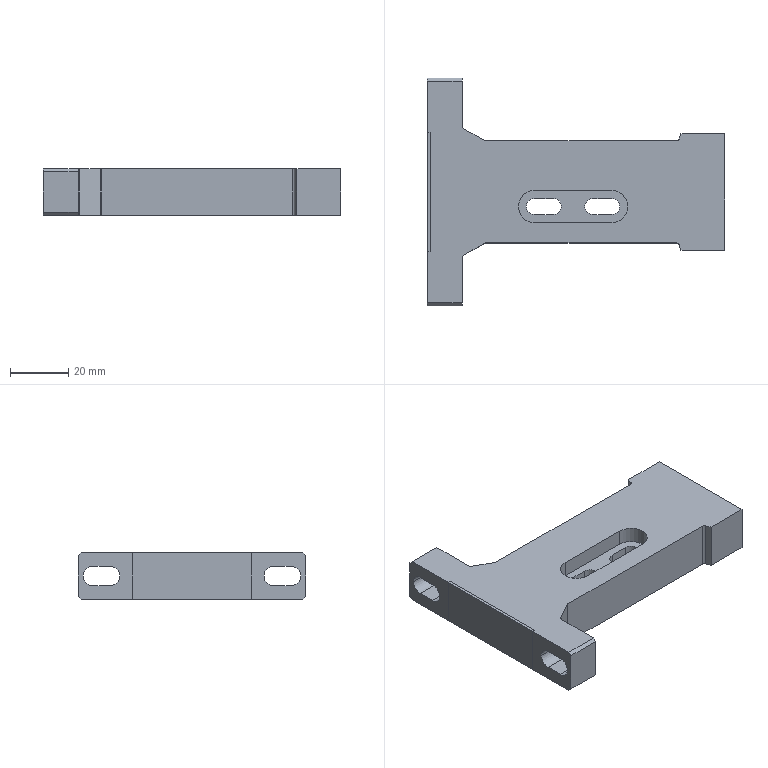NC program | NX | posted with a generic post | part box 102 x 78 x 16 mm
Lines 2465 to 2749 of 11044:
(ZLEVEL_PROFILE_COPY_COPY_1 , TOOL : D10JING)
N4922 T11 M6
N4924 G54
N4926 G17 G0 G90 X-56.438 Y-39.827 B0. C0. S9500 M3
N4928 G43 Z30. H11
N4930 Z-13.
N4932 G94 G1 Z-16. F1200.
N4934 G3 X-56. Y-39. R1.
N4936 G1 Y39.
N4938 G2 X-51. Y44. R5.
N4940 G1 X-39.
N4942 G2 X-34. Y39. R5.
N4944 G1 Y24.887
N4946 X-29.866 Y22.5
N4948 X31.67
N4950 G2 X36. Y25. R5.
N4952 G1 X51.
N4954 G2 X56. Y20. R5.
N4956 G1 Y-20.
N4958 G2 X51. Y-25. R5.
N4960 G1 X36.
N4962 G2 X31.67 Y-22.5 R5.
N4964 G1 X-29.866
N4966 X-34. Y-24.887
N4968 Y-39.
N4970 G2 X-39. Y-44. R5.
N4972 G1 X-51.
N4974 G2 X-56. Y-39. R5.
N4976 G3 X-56.5 Y-38.134 R1.
N4978 G1 Z-13.
N4980 G0 Z30.
N4982 M5
(ZLEVEL_PROFILE_COPY_COPY_1_COPY_1 , TOOL : D6)
N4984 T06 M6
N4986 G54
N4988 G17 G0 G90 X14.695 Y-5.095 B0. C0. S9500 M3
N4990 G43 Z30. H6
N4992 Z1.5
N4994 G94 G1 X14.691 Y-4.699 Z1.479 F2200.
N4996 X14.559 Y-4.152 Z1.45
N4998 X14.37 Y-3.752 Z1.427
N5000 X14.017 Y-3.289 Z1.396
N5002 X13.566 Y-2.921 Z1.366
N5004 X13.041 Y-2.671 Z1.335
N5006 X12.472 Y-2.55 Z1.305
N5008 X-14.472 Z-0.107
N5010 X-15.041 Y-2.671 Z-0.138
N5012 X-15.566 Y-2.921 Z-0.168
N5014 X-16.017 Y-3.289 Z-0.199
N5016 X-16.37 Y-3.752 Z-0.229
N5018 X-16.559 Y-4.152 Z-0.253
N5020 X-16.691 Y-4.699 Z-0.282
N5022 X-16.696 Y-5.261 Z-0.312
N5024 X-16.573 Y-5.809 Z-0.341
N5026 X-16.329 Y-6.316 Z-0.371
N5028 X-15.975 Y-6.753 Z-0.4
N5030 X-15.532 Y-7.099 Z-0.429
N5032 X-15.022 Y-7.336 Z-0.459
N5034 X-14.472 Y-7.45 Z-0.488
N5036 X-14.25 Z-0.5
N5038 X12.25
N5040 G3 X14.7 Y-5. R2.45
N5042 X12.25 Y-2.55 R2.45
N5044 G1 X-14.25
N5046 G3 X-16.7 Y-5. R2.45
N5048 X-14.25 Y-7.45 R2.45
N5050 G1 X11.979 Z-0.958
N5052 X12.152 Z-0.961
N5054 X12.324 Y-7.44 Z-0.964
N5056 X12.496 Y-7.431 Z-0.967
N5058 X12.666 Y-7.406 Z-0.97
N5060 X12.835 Y-7.373 Z-0.973
N5062 X13. Y-7.324 Z-0.976
N5064 X13.162 Y-7.266 Z-0.979
N5066 X13.32 Y-7.198 Z-0.982
N5068 X13.47 Y-7.114 Z-0.985
N5070 X13.618 Y-7.026 Z-0.988
N5072 X13.755 Y-6.923 Z-0.991
N5074 X13.887 Y-6.812 Z-0.994
N5076 X14.012 Y-6.693 Z-0.997
N5078 X14.131 Y-6.569 Z-1.
N5080 G3 X12.25 Y-2.55 R2.45
N5082 G1 X-14.25
N5084 G3 X-16.7 Y-5. R2.45
N5086 X-14.25 Y-7.45 R2.45
N5088 G1 X11.979 Z-1.458
N5090 X12.152 Z-1.461
N5092 X12.324 Y-7.44 Z-1.464
N5094 X12.496 Y-7.431 Z-1.467
N5096 X12.666 Y-7.406 Z-1.47
N5098 X12.835 Y-7.373 Z-1.473
N5100 X13. Y-7.323 Z-1.476
N5102 X13.161 Y-7.265 Z-1.479
N5104 X13.319 Y-7.198 Z-1.482
N5106 X13.47 Y-7.114 Z-1.485
N5108 X13.617 Y-7.026 Z-1.488
N5110 X13.755 Y-6.923 Z-1.491
N5112 X13.886 Y-6.812 Z-1.494
N5114 X14.012 Y-6.693 Z-1.497
N5116 X14.131 Y-6.569 Z-1.5
N5118 G3 X12.25 Y-2.55 R2.45
N5120 G1 X-14.25
N5122 G3 X-16.7 Y-5. R2.45
N5124 X-14.25 Y-7.45 R2.45
N5126 G1 X11.979 Z-1.958
N5128 X12.152 Z-1.961
N5130 X12.324 Y-7.44 Z-1.964
N5132 X12.496 Y-7.431 Z-1.967
N5134 X12.666 Y-7.406 Z-1.97
N5136 X12.835 Y-7.372 Z-1.973
N5138 X12.999 Y-7.323 Z-1.976
N5140 X13.161 Y-7.265 Z-1.979
N5142 X13.319 Y-7.198 Z-1.982
N5144 X13.47 Y-7.114 Z-1.985
N5146 X13.617 Y-7.026 Z-1.988
N5148 X13.755 Y-6.923 Z-1.991
N5150 X13.886 Y-6.812 Z-1.994
N5152 X14.012 Y-6.693 Z-1.997
N5154 X14.131 Y-6.569 Z-2.
N5156 G3 X12.25 Y-2.55 R2.45
N5158 G1 X-14.25
N5160 G3 X-16.7 Y-5. R2.45
N5162 X-14.25 Y-7.45 R2.45
N5164 G1 X11.979 Z-2.458
N5166 X12.152 Z-2.461
N5168 X12.324 Y-7.44 Z-2.464
N5170 X12.496 Y-7.431 Z-2.467
N5172 X12.666 Y-7.405 Z-2.47
N5174 X12.835 Y-7.372 Z-2.473
N5176 X12.999 Y-7.323 Z-2.476
N5178 X13.161 Y-7.265 Z-2.479
N5180 X13.319 Y-7.197 Z-2.482
N5182 X13.469 Y-7.113 Z-2.485
N5184 X13.617 Y-7.026 Z-2.488
N5186 X13.755 Y-6.923 Z-2.491
N5188 X13.886 Y-6.812 Z-2.494
N5190 X14.011 Y-6.693 Z-2.497
N5192 X14.131 Y-6.569 Z-2.5
N5194 G3 X12.25 Y-2.55 R2.45
N5196 G1 X-14.25
N5198 G3 X-16.7 Y-5. R2.45
N5200 X-14.25 Y-7.45 R2.45
N5202 G1 X11.979 Z-2.958
N5204 X12.152 Z-2.961
N5206 X12.324 Y-7.44 Z-2.964
N5208 X12.496 Y-7.43 Z-2.967
N5210 X12.666 Y-7.405 Z-2.97
N5212 X12.834 Y-7.372 Z-2.973
N5214 X12.999 Y-7.323 Z-2.976
N5216 X13.161 Y-7.265 Z-2.979
N5218 X13.319 Y-7.197 Z-2.982
N5220 X13.47 Y-7.114 Z-2.985
N5222 X13.617 Y-7.025 Z-2.988
N5224 X13.755 Y-6.922 Z-2.991
N5226 X13.886 Y-6.811 Z-2.994
N5228 X14.011 Y-6.693 Z-2.997
N5230 X14.131 Y-6.569 Z-3.
N5232 G3 X12.25 Y-2.55 R2.45
N5234 G1 X-14.25
N5236 G3 X-16.7 Y-5. R2.45
N5238 X-14.25 Y-7.45 R2.45
N5240 G1 X11.979 Z-3.458
N5242 X12.152 Z-3.461
N5244 X12.324 Y-7.44 Z-3.464
N5246 X12.496 Y-7.43 Z-3.467
N5248 X12.666 Y-7.405 Z-3.47
N5250 X12.835 Y-7.373 Z-3.473
N5252 X12.999 Y-7.323 Z-3.476
N5254 X13.161 Y-7.265 Z-3.479
N5256 X13.319 Y-7.197 Z-3.482
N5258 X13.47 Y-7.114 Z-3.485
N5260 X13.617 Y-7.025 Z-3.488
N5262 X13.755 Y-6.922 Z-3.491
N5264 X13.886 Y-6.811 Z-3.494
N5266 X14.011 Y-6.693 Z-3.497
N5268 X14.131 Y-6.569 Z-3.5
N5270 G3 X12.25 Y-2.55 R2.45
N5272 G1 X-14.25
N5274 G3 X-16.7 Y-5. R2.45
N5276 X-14.25 Y-7.45 R2.45
N5278 G1 X11.979 Z-3.958
N5280 X12.152 Z-3.961
N5282 X12.324 Y-7.44 Z-3.964
N5284 X12.496 Y-7.43 Z-3.967
N5286 X12.666 Y-7.405 Z-3.97
N5288 X12.835 Y-7.373 Z-3.973
N5290 X12.999 Y-7.323 Z-3.976
N5292 X13.161 Y-7.264 Z-3.979
N5294 X13.319 Y-7.197 Z-3.982
N5296 X13.47 Y-7.114 Z-3.985
N5298 X13.617 Y-7.025 Z-3.988
N5300 X13.755 Y-6.922 Z-3.991
N5302 X13.886 Y-6.811 Z-3.994
N5304 X14.011 Y-6.693 Z-3.997
N5306 X14.131 Y-6.569 Z-4.
N5308 G3 X12.25 Y-2.55 R2.45
N5310 G1 X-14.25
N5312 G3 X-16.7 Y-5. R2.45
N5314 X-14.25 Y-7.45 R2.45
N5316 G1 X11.979 Z-4.458
N5318 X12.152 Z-4.461
N5320 X12.324 Y-7.44 Z-4.464
N5322 X12.496 Y-7.43 Z-4.467
N5324 X12.666 Y-7.405 Z-4.47
N5326 X12.835 Y-7.373 Z-4.473
N5328 X12.999 Y-7.323 Z-4.476
N5330 X13.161 Y-7.264 Z-4.479
N5332 X13.319 Y-7.197 Z-4.482
N5334 X13.47 Y-7.114 Z-4.485
N5336 X13.617 Y-7.025 Z-4.488
N5338 X13.754 Y-6.922 Z-4.491
N5340 X13.886 Y-6.811 Z-4.494
N5342 X14.011 Y-6.693 Z-4.497
N5344 X14.131 Y-6.569 Z-4.5
N5346 G3 X12.25 Y-2.55 R2.45
N5348 G1 X-14.25
N5350 G3 X-16.7 Y-5. R2.45
N5352 X-14.25 Y-7.45 R2.45
N5354 G1 X11.979 Z-4.958
N5356 X12.152 Z-4.961
N5358 X12.324 Y-7.439 Z-4.964
N5360 X12.496 Y-7.43 Z-4.967
N5362 X12.666 Y-7.405 Z-4.97
N5364 X12.835 Y-7.372 Z-4.973
N5366 X12.999 Y-7.323 Z-4.976
N5368 X13.161 Y-7.264 Z-4.979
N5370 X13.319 Y-7.197 Z-4.982
N5372 X13.47 Y-7.114 Z-4.985
N5374 X13.617 Y-7.025 Z-4.988
N5376 X13.754 Y-6.922 Z-4.991
N5378 X13.886 Y-6.811 Z-4.994
N5380 X14.012 Y-6.693 Z-4.997
N5382 X14.131 Y-6.569 Z-5.
N5384 G3 X12.25 Y-2.55 R2.45
N5386 G1 X-14.25
N5388 G3 X-16.7 Y-5. R2.45
N5390 X-14.25 Y-7.45 R2.45
N5392 G1 X11.979 Z-5.458
N5394 X12.152 Z-5.461
N5396 X12.324 Y-7.439 Z-5.464
N5398 X12.496 Y-7.429 Z-5.467
N5400 X12.666 Y-7.405 Z-5.47
N5402 X12.835 Y-7.372 Z-5.473
N5404 X12.999 Y-7.323 Z-5.476
N5406 X13.161 Y-7.264 Z-5.479
N5408 X13.319 Y-7.197 Z-5.482
N5410 X13.469 Y-7.113 Z-5.485
N5412 X13.617 Y-7.025 Z-5.488
N5414 X13.754 Y-6.921 Z-5.491
N5416 X13.886 Y-6.811 Z-5.494
N5418 X14.012 Y-6.693 Z-5.497
N5420 X14.131 Y-6.569 Z-5.5
N5422 G3 X12.25 Y-2.55 R2.45
N5424 G1 X-14.25
N5426 G3 X-16.7 Y-5. R2.45
N5428 X-14.25 Y-7.45 R2.45
N5430 G1 X12.25
N5432 G3 X14.131 Y-6.569 R2.45
N5434 X14.234 Y-5.978 R0.6
N5436 G1 X14.1 Y-5.615
N5438 Z-4.9
N5440 G0 Z30.
(ZLEVEL_PROFILE_COPY_COPY_1_COPY_2 , TOOL : D6)
N5442 X-14.96 Y-6.87
N5444 Z-2.5
N5446 G1 Z-5.5 F1200.
N5448 X-14.77 Y-7.2
N5450 G3 X-14.25 Y-7.5 R0.6
N5452 G1 X12.25
N5454 G3 X14.75 Y-5. R2.5
N5456 X12.25 Y-2.5 R2.5
N5458 G1 X-14.25
N5460 G3 X-16.75 Y-5. R2.5
N5462 X-14.25 Y-7.5 R2.5
N5464 X-13.73 Y-7.2 R0.6
N5466 G1 X-13.615 Y-7.
N5468 Z-2.5
N5470 G0 Z30.
N5472 M5